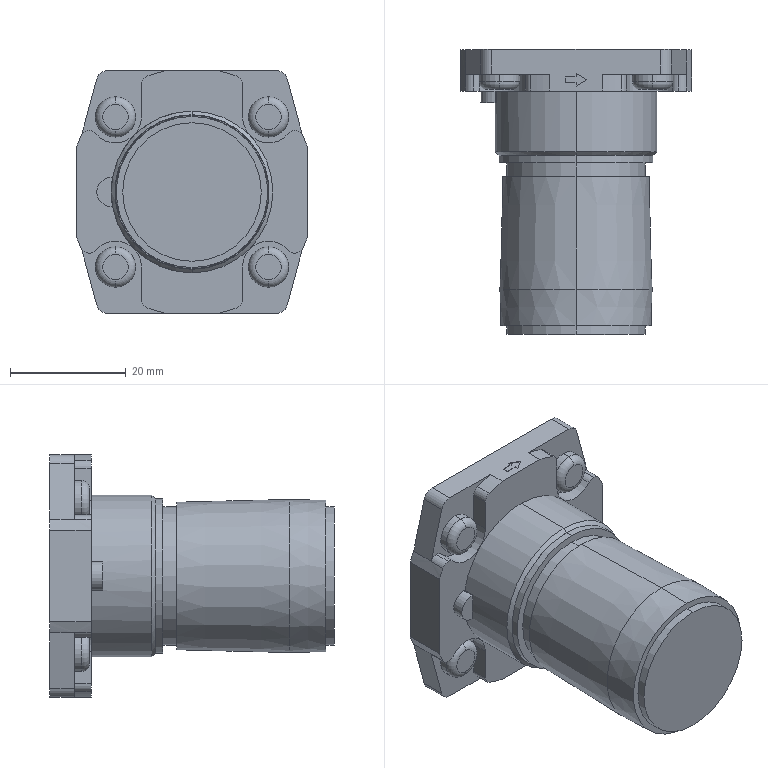Part | STEP file | 25A-AR20K-01B-D-Part-4 | 1 solid | 105 faces | box 40 x 49.3 x 42 mm | volume 33597 mm3 | cylinder 47 | plane 44 | torus 8 | cone 6 | commonest cylinder face diameters 3 x10 7 x8 43 x8 9 x6 4 x4 24 x4